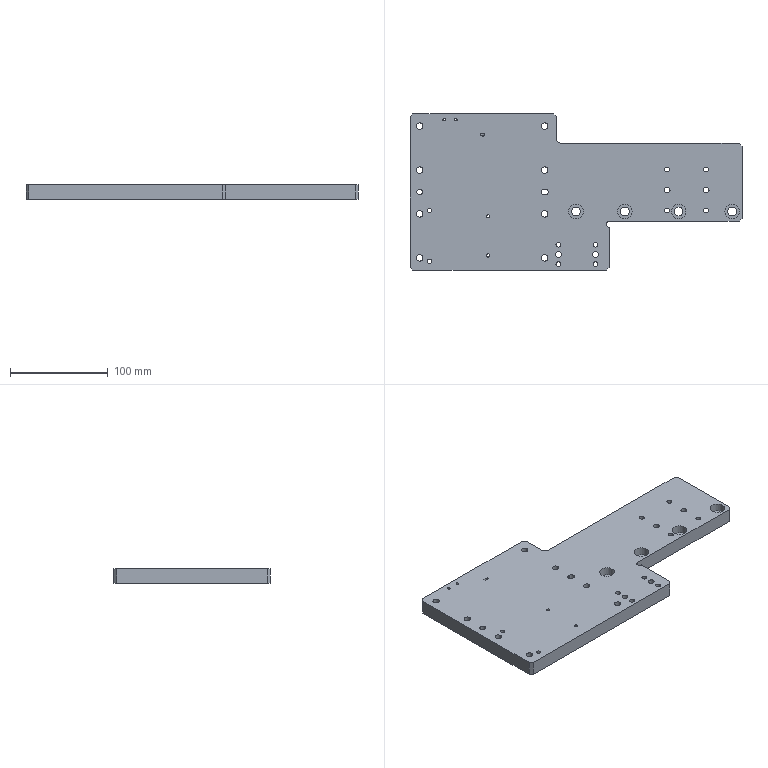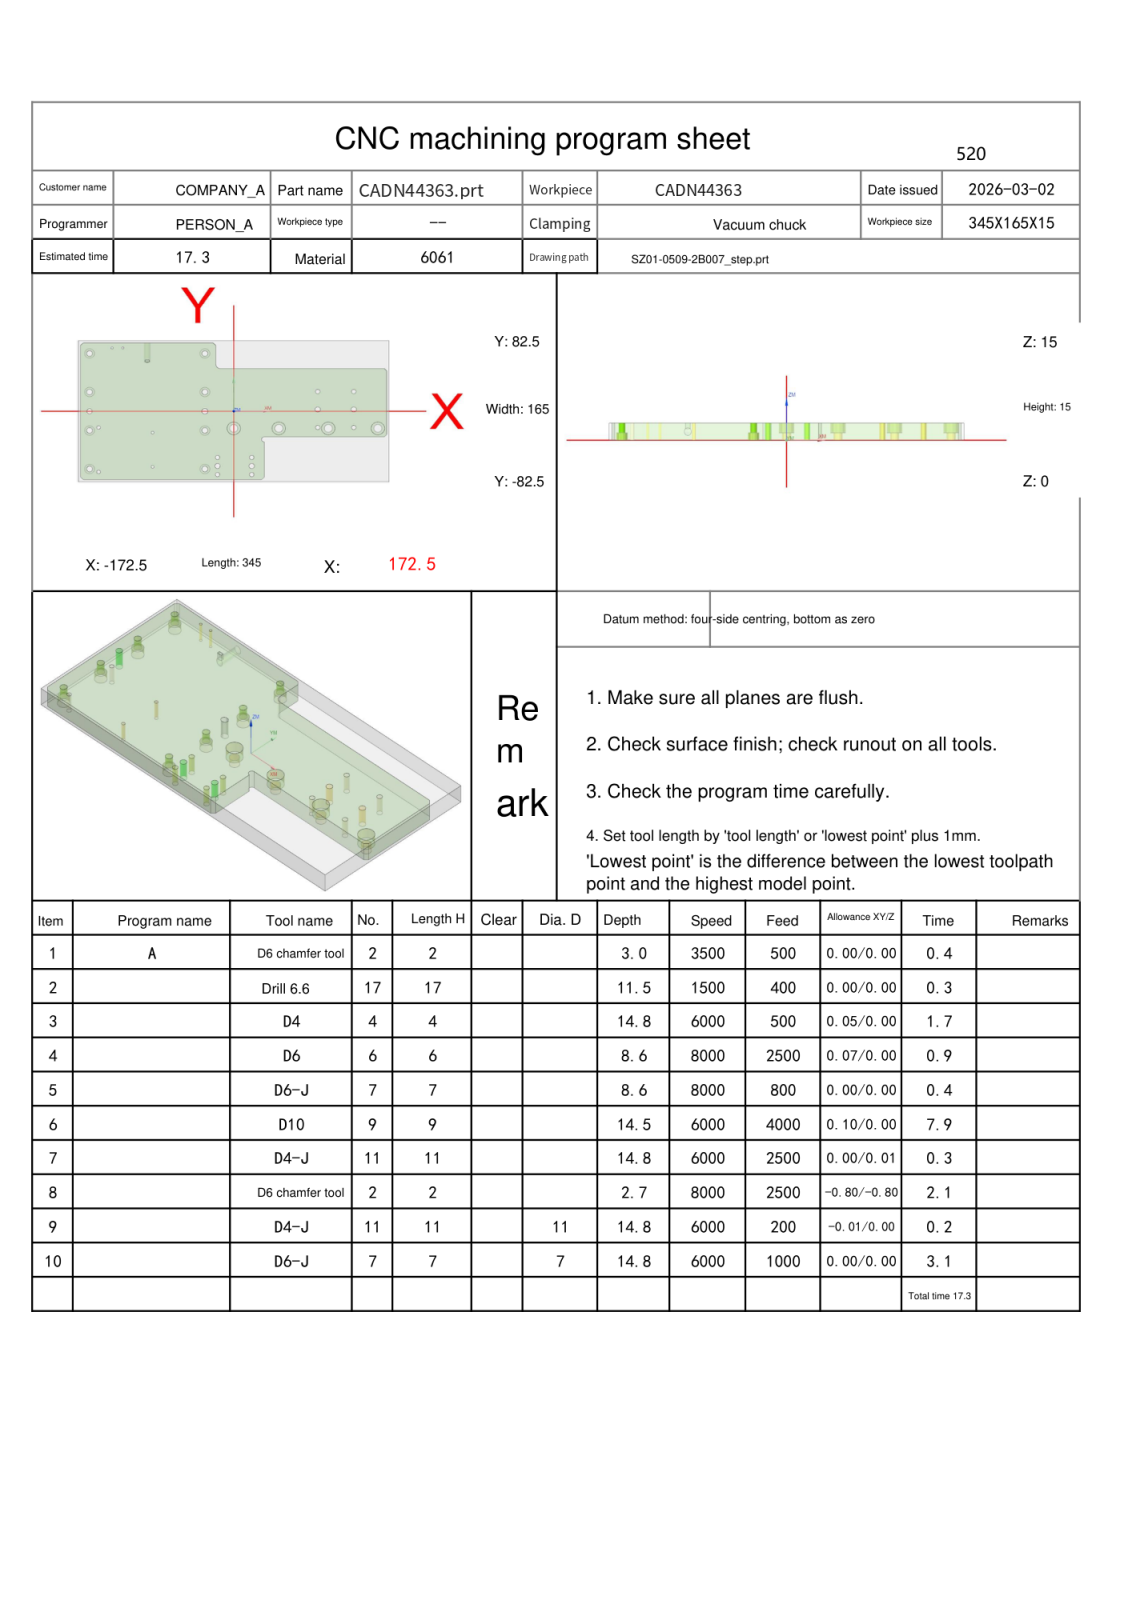NC program | NX | posted by the shop | part box 340 x 160 x 15 mm
Lines 1831 to 3961 of 3961, first 1633 of 2131 lines:
N7 T11 M06
(D4-J  D=4. R=0. H=11 ce=0.00 di=0.01)
G00 G90 G54 X39.452 Y-32.6 M03 S6000
G43 H11 Z65.
M08
Z15.304
G01 X39.451 Y-32.593 Z15.218 F2000.
X39.448 Y-32.574 Z15.14
X39.443 Y-32.545 Z15.07
X39.434 Y-32.506 Z15.008
X39.424 Y-32.461 Z14.952
X39.41 Y-32.41 Z14.903
X39.393 Y-32.356 Z14.861
X39.372 Y-32.3 Z14.824
X39.348 Y-32.244 Z14.793
X39.319 Y-32.19 Z14.767
X39.287 Y-32.139 Z14.746
X39.249 Y-32.094 Z14.73
X39.208 Y-32.055 Z14.718
X39.161 Y-32.026 Z14.71
X39.109 Y-32.007 Z14.705
X39.052 Y-32. Z14.704
X34. F2500.
G03 X33. Y-33. I0.0 J-1.
X34. Y-34. I1. J0.0
G02 X35.996 Y-35.879 I0.0 J-2.
G01 X36.015 Y-35.919 Z14.703
X36.063 Y-35.933 Z14.701
X36.136 Y-35.922 Z14.696
X36.231 Y-35.888 Z14.691
X36.344 Y-35.834 Z14.684
X36.473 Y-35.762 Z14.676
X36.615 Y-35.674 Z14.667
X36.765 Y-35.572 Z14.657
X37.001 Y-35.394 Z14.641
X37.233 Y-35.202 Z14.624
X37.561 Y-34.893 Z14.597
X37.866 Y-34.56 Z14.57
X38.147 Y-34.204 Z14.542
X38.404 Y-33.826 Z14.515
X38.635 Y-33.429 Z14.488
X38.774 Y-33.153 Z14.471
X38.858 Y-32.97 Z14.46
X38.971 Y-32.701 Z14.445
X39.03 Y-32.537 Z14.436
X39.076 Y-32.388 Z14.428
X39.107 Y-32.259 Z14.421
X39.121 Y-32.151 Z14.416
X39.118 Y-32.07 Z14.411
X39.096 Y-32.018 Z14.409
X39.052 Y-32. Z14.408
X34.
G03 X33. Y-33. I0.0 J-1.
X34. Y-34. I1. J0.0
G02 X35.996 Y-35.879 I0.0 J-2.
G01 X36.015 Y-35.919 Z14.407
X36.063 Y-35.933 Z14.405
X36.136 Y-35.922 Z14.4
X36.231 Y-35.888 Z14.395
X36.344 Y-35.834 Z14.388
X36.473 Y-35.762 Z14.38
X36.615 Y-35.674 Z14.371
X36.765 Y-35.572 Z14.361
X37.001 Y-35.394 Z14.345
X37.233 Y-35.202 Z14.328
X37.561 Y-34.893 Z14.301
X37.866 Y-34.56 Z14.274
X38.147 Y-34.204 Z14.246
X38.404 Y-33.826 Z14.219
X38.635 Y-33.429 Z14.192
X38.774 Y-33.153 Z14.175
X38.858 Y-32.97 Z14.164
X38.971 Y-32.701 Z14.149
X39.03 Y-32.537 Z14.14
X39.076 Y-32.388 Z14.132
X39.107 Y-32.259 Z14.125
X39.121 Y-32.151 Z14.12
X39.118 Y-32.07 Z14.115
X39.096 Y-32.018 Z14.113
X39.052 Y-32. Z14.112
X34.
G03 X33. Y-33. I0.0 J-1.
X34. Y-34. I1. J0.0
G02 X35.996 Y-35.879 I0.0 J-2.
G01 X36.015 Y-35.919 Z14.111
X36.063 Y-35.933 Z14.109
X36.136 Y-35.922 Z14.104
X36.231 Y-35.888 Z14.099
X36.344 Y-35.834 Z14.092
X36.473 Y-35.762 Z14.084
X36.615 Y-35.674 Z14.075
X36.765 Y-35.572 Z14.065
X37.001 Y-35.394 Z14.049
X37.233 Y-35.202 Z14.032
X37.561 Y-34.893 Z14.005
X37.866 Y-34.56 Z13.978
X38.147 Y-34.204 Z13.95
X38.404 Y-33.826 Z13.923
X38.635 Y-33.429 Z13.896
X38.774 Y-33.153 Z13.879
X38.858 Y-32.97 Z13.868
X38.971 Y-32.701 Z13.853
X39.03 Y-32.537 Z13.844
X39.076 Y-32.388 Z13.836
X39.107 Y-32.259 Z13.829
X39.121 Y-32.151 Z13.824
X39.118 Y-32.07 Z13.819
X39.096 Y-32.018 Z13.817
X39.052 Y-32. Z13.816
X34.
G03 X33. Y-33. I0.0 J-1.
X34. Y-34. I1. J0.0
G02 X35.996 Y-35.879 I0.0 J-2.
G01 X36.015 Y-35.919 Z13.815
X36.063 Y-35.933 Z13.813
X36.136 Y-35.922 Z13.808
X36.231 Y-35.888 Z13.803
X36.344 Y-35.834 Z13.796
X36.473 Y-35.762 Z13.788
X36.615 Y-35.674 Z13.779
X36.765 Y-35.572 Z13.769
X37.001 Y-35.394 Z13.753
X37.233 Y-35.202 Z13.736
X37.561 Y-34.893 Z13.709
X37.866 Y-34.56 Z13.682
X38.147 Y-34.204 Z13.654
X38.404 Y-33.826 Z13.627
X38.635 Y-33.429 Z13.6
X38.774 Y-33.153 Z13.583
X38.858 Y-32.97 Z13.572
X38.971 Y-32.701 Z13.557
X39.03 Y-32.537 Z13.548
X39.076 Y-32.388 Z13.54
X39.107 Y-32.259 Z13.533
X39.121 Y-32.151 Z13.528
X39.118 Y-32.07 Z13.523
X39.096 Y-32.018 Z13.521
X39.052 Y-32. Z13.52
X34.
G03 X33. Y-33. I0.0 J-1.
X34. Y-34. I1. J0.0
G02 X35.996 Y-35.879 I0.0 J-2.
G01 X36.015 Y-35.919 Z13.519
X36.063 Y-35.933 Z13.517
X36.136 Y-35.922 Z13.512
X36.231 Y-35.888 Z13.507
X36.344 Y-35.834 Z13.5
X36.473 Y-35.762 Z13.492
X36.615 Y-35.674 Z13.483
X36.765 Y-35.572 Z13.473
X37.001 Y-35.394 Z13.457
X37.233 Y-35.202 Z13.44
X37.561 Y-34.893 Z13.413
X37.866 Y-34.56 Z13.386
X38.147 Y-34.204 Z13.358
X38.404 Y-33.826 Z13.331
X38.635 Y-33.429 Z13.304
X38.774 Y-33.153 Z13.287
X38.858 Y-32.97 Z13.276
X38.971 Y-32.701 Z13.261
X39.03 Y-32.537 Z13.252
X39.076 Y-32.388 Z13.244
X39.107 Y-32.259 Z13.237
X39.121 Y-32.151 Z13.232
X39.118 Y-32.07 Z13.227
X39.096 Y-32.018 Z13.225
X39.052 Y-32. Z13.224
X34.
G03 X33. Y-33. I0.0 J-1.
X34. Y-34. I1. J0.0
G02 X35.996 Y-35.879 I0.0 J-2.
G01 X36.015 Y-35.919 Z13.223
X36.063 Y-35.933 Z13.221
X36.136 Y-35.922 Z13.216
X36.231 Y-35.888 Z13.211
X36.344 Y-35.834 Z13.204
X36.473 Y-35.762 Z13.196
X36.615 Y-35.674 Z13.187
X36.765 Y-35.572 Z13.177
X37.001 Y-35.394 Z13.161
X37.233 Y-35.202 Z13.144
X37.561 Y-34.893 Z13.117
X37.866 Y-34.56 Z13.09
X38.147 Y-34.204 Z13.062
X38.404 Y-33.826 Z13.035
X38.635 Y-33.429 Z13.008
X38.774 Y-33.153 Z12.991
X38.858 Y-32.97 Z12.98
X38.971 Y-32.701 Z12.965
X39.03 Y-32.537 Z12.956
X39.076 Y-32.388 Z12.948
X39.107 Y-32.259 Z12.941
X39.121 Y-32.151 Z12.936
X39.118 Y-32.07 Z12.931
X39.096 Y-32.018 Z12.929
X39.052 Y-32. Z12.928
X34.
G03 X33. Y-33. I0.0 J-1.
X34. Y-34. I1. J0.0
G02 X35.996 Y-35.879 I0.0 J-2.
G01 X36.015 Y-35.919 Z12.927
X36.063 Y-35.933 Z12.925
X36.136 Y-35.922 Z12.92
X36.231 Y-35.888 Z12.915
X36.344 Y-35.834 Z12.908
X36.473 Y-35.762 Z12.9
X36.615 Y-35.674 Z12.891
X36.765 Y-35.572 Z12.881
X37.001 Y-35.394 Z12.865
X37.233 Y-35.202 Z12.848
X37.561 Y-34.893 Z12.821
X37.866 Y-34.56 Z12.794
X38.147 Y-34.204 Z12.766
X38.404 Y-33.826 Z12.739
X38.635 Y-33.429 Z12.712
X38.774 Y-33.153 Z12.695
X38.858 Y-32.97 Z12.684
X38.971 Y-32.701 Z12.669
X39.03 Y-32.537 Z12.66
X39.076 Y-32.388 Z12.652
X39.107 Y-32.259 Z12.645
X39.121 Y-32.151 Z12.64
X39.118 Y-32.07 Z12.635
X39.096 Y-32.018 Z12.633
X39.052 Y-32. Z12.632
X34.
G03 X33. Y-33. I0.0 J-1.
X34. Y-34. I1. J0.0
G02 X35.996 Y-35.879 I0.0 J-2.
G01 X36.015 Y-35.919 Z12.631
X36.063 Y-35.933 Z12.629
X36.136 Y-35.922 Z12.624
X36.231 Y-35.888 Z12.619
X36.344 Y-35.834 Z12.612
X36.473 Y-35.762 Z12.604
X36.615 Y-35.674 Z12.595
X36.765 Y-35.572 Z12.585
X37.001 Y-35.394 Z12.569
X37.233 Y-35.202 Z12.552
X37.561 Y-34.893 Z12.525
X37.866 Y-34.56 Z12.498
X38.147 Y-34.204 Z12.47
X38.404 Y-33.826 Z12.443
X38.635 Y-33.429 Z12.416
X38.774 Y-33.153 Z12.399
X38.858 Y-32.97 Z12.388
X38.971 Y-32.701 Z12.373
X39.03 Y-32.537 Z12.364
X39.076 Y-32.388 Z12.356
X39.107 Y-32.259 Z12.349
X39.121 Y-32.151 Z12.344
X39.118 Y-32.07 Z12.339
X39.096 Y-32.018 Z12.337
X39.052 Y-32. Z12.336
X34.
G03 X33. Y-33. I0.0 J-1.
X34. Y-34. I1. J0.0
G02 X35.996 Y-35.879 I0.0 J-2.
G01 X36.015 Y-35.919 Z12.335
X36.063 Y-35.933 Z12.333
X36.136 Y-35.922 Z12.328
X36.231 Y-35.888 Z12.323
X36.344 Y-35.834 Z12.316
X36.473 Y-35.762 Z12.308
X36.615 Y-35.674 Z12.299
X36.765 Y-35.572 Z12.289
X37.001 Y-35.394 Z12.273
X37.233 Y-35.202 Z12.256
X37.561 Y-34.893 Z12.229
X37.866 Y-34.56 Z12.202
X38.147 Y-34.204 Z12.174
X38.404 Y-33.826 Z12.147
X38.635 Y-33.429 Z12.12
X38.774 Y-33.153 Z12.103
X38.858 Y-32.97 Z12.092
X38.971 Y-32.701 Z12.077
X39.03 Y-32.537 Z12.068
X39.076 Y-32.388 Z12.06
X39.107 Y-32.259 Z12.053
X39.121 Y-32.151 Z12.048
X39.118 Y-32.07 Z12.043
X39.096 Y-32.018 Z12.041
X39.052 Y-32. Z12.04
X34.
G03 X33. Y-33. I0.0 J-1.
X34. Y-34. I1. J0.0
G02 X35.996 Y-35.879 I0.0 J-2.
G01 X36.015 Y-35.919 Z12.039
X36.063 Y-35.933 Z12.037
X36.136 Y-35.922 Z12.032
X36.231 Y-35.888 Z12.027
X36.344 Y-35.834 Z12.02
X36.473 Y-35.762 Z12.012
X36.615 Y-35.674 Z12.003
X36.765 Y-35.572 Z11.993
X37.001 Y-35.394 Z11.977
X37.233 Y-35.202 Z11.96
X37.561 Y-34.893 Z11.933
X37.866 Y-34.56 Z11.906
X38.147 Y-34.204 Z11.878
X38.404 Y-33.826 Z11.851
X38.635 Y-33.429 Z11.824
X38.774 Y-33.153 Z11.807
X38.858 Y-32.97 Z11.796
X38.971 Y-32.701 Z11.781
X39.03 Y-32.537 Z11.772
X39.076 Y-32.388 Z11.764
X39.107 Y-32.259 Z11.757
X39.121 Y-32.151 Z11.752
X39.118 Y-32.07 Z11.747
X39.096 Y-32.018 Z11.745
X39.052 Y-32. Z11.744
X34.
G03 X33. Y-33. I0.0 J-1.
X34. Y-34. I1. J0.0
G02 X35.996 Y-35.879 I0.0 J-2.
G01 X36.015 Y-35.919 Z11.743
X36.063 Y-35.933 Z11.741
X36.136 Y-35.922 Z11.736
X36.231 Y-35.888 Z11.731
X36.344 Y-35.834 Z11.724
X36.473 Y-35.762 Z11.716
X36.615 Y-35.674 Z11.707
X36.765 Y-35.572 Z11.697
X37.001 Y-35.394 Z11.681
X37.233 Y-35.202 Z11.664
X37.561 Y-34.893 Z11.637
X37.866 Y-34.56 Z11.61
X38.147 Y-34.204 Z11.582
X38.404 Y-33.826 Z11.555
X38.635 Y-33.429 Z11.528
X38.774 Y-33.153 Z11.511
X38.858 Y-32.97 Z11.5
X38.971 Y-32.701 Z11.485
X39.03 Y-32.537 Z11.476
X39.076 Y-32.388 Z11.468
X39.107 Y-32.259 Z11.461
X39.121 Y-32.151 Z11.456
X39.118 Y-32.07 Z11.451
X39.096 Y-32.018 Z11.449
X39.052 Y-32. Z11.448
X34.
G03 X33. Y-33. I0.0 J-1.
X34. Y-34. I1. J0.0
G02 X35.996 Y-35.879 I0.0 J-2.
G01 X36.015 Y-35.919 Z11.447
X36.063 Y-35.933 Z11.445
X36.136 Y-35.922 Z11.44
X36.231 Y-35.888 Z11.435
X36.344 Y-35.834 Z11.428
X36.473 Y-35.762 Z11.42
X36.615 Y-35.674 Z11.411
X36.765 Y-35.572 Z11.401
X37.001 Y-35.394 Z11.385
X37.233 Y-35.202 Z11.368
X37.561 Y-34.893 Z11.341
X37.866 Y-34.56 Z11.314
X38.147 Y-34.204 Z11.286
X38.404 Y-33.826 Z11.259
X38.635 Y-33.429 Z11.232
X38.774 Y-33.153 Z11.215
X38.858 Y-32.97 Z11.204
X38.971 Y-32.701 Z11.189
X39.03 Y-32.537 Z11.18
X39.076 Y-32.388 Z11.172
X39.107 Y-32.259 Z11.165
X39.121 Y-32.151 Z11.16
X39.118 Y-32.07 Z11.155
X39.096 Y-32.018 Z11.153
X39.052 Y-32. Z11.152
X34.
G03 X33. Y-33. I0.0 J-1.
X34. Y-34. I1. J0.0
G02 X35.996 Y-35.879 I0.0 J-2.
G01 X36.015 Y-35.919 Z11.151
X36.063 Y-35.933 Z11.149
X36.136 Y-35.922 Z11.144
X36.231 Y-35.888 Z11.139
X36.344 Y-35.834 Z11.132
X36.473 Y-35.762 Z11.124
X36.615 Y-35.674 Z11.115
X36.765 Y-35.572 Z11.105
X37.001 Y-35.394 Z11.089
X37.233 Y-35.202 Z11.072
X37.561 Y-34.893 Z11.045
X37.866 Y-34.56 Z11.018
X38.147 Y-34.204 Z10.99
X38.404 Y-33.826 Z10.963
X38.635 Y-33.429 Z10.936
X38.774 Y-33.153 Z10.919
X38.858 Y-32.97 Z10.908
X38.971 Y-32.701 Z10.893
X39.03 Y-32.537 Z10.884
X39.076 Y-32.388 Z10.876
X39.107 Y-32.259 Z10.869
X39.121 Y-32.151 Z10.864
X39.118 Y-32.07 Z10.859
X39.096 Y-32.018 Z10.857
X39.052 Y-32. Z10.856
X34.
G03 X33. Y-33. I0.0 J-1.
X34. Y-34. I1. J0.0
G02 X35.996 Y-35.879 I0.0 J-2.
G01 X36.015 Y-35.919 Z10.855
X36.063 Y-35.933 Z10.853
X36.136 Y-35.922 Z10.848
X36.231 Y-35.888 Z10.843
X36.344 Y-35.834 Z10.836
X36.473 Y-35.762 Z10.828
X36.615 Y-35.674 Z10.819
X36.765 Y-35.572 Z10.809
X37.001 Y-35.394 Z10.793
X37.233 Y-35.202 Z10.776
X37.561 Y-34.893 Z10.749
X37.866 Y-34.56 Z10.722
X38.147 Y-34.204 Z10.694
X38.404 Y-33.826 Z10.667
X38.635 Y-33.429 Z10.64
X38.774 Y-33.153 Z10.623
X38.858 Y-32.97 Z10.612
X38.971 Y-32.701 Z10.597
X39.03 Y-32.537 Z10.588
X39.076 Y-32.388 Z10.58
X39.107 Y-32.259 Z10.573
X39.121 Y-32.151 Z10.568
X39.118 Y-32.07 Z10.563
X39.096 Y-32.018 Z10.561
X39.052 Y-32. Z10.56
X34.
G03 X33. Y-33. I0.0 J-1.
X34. Y-34. I1. J0.0
G02 X35.996 Y-35.879 I0.0 J-2.
G01 X36.015 Y-35.919 Z10.559
X36.063 Y-35.933 Z10.557
X36.136 Y-35.922 Z10.552
X36.231 Y-35.888 Z10.547
X36.344 Y-35.834 Z10.54
X36.473 Y-35.762 Z10.532
X36.615 Y-35.674 Z10.523
X36.765 Y-35.572 Z10.513
X37.001 Y-35.394 Z10.497
X37.233 Y-35.202 Z10.48
X37.561 Y-34.893 Z10.453
X37.866 Y-34.56 Z10.426
X38.147 Y-34.204 Z10.398
X38.404 Y-33.826 Z10.371
X38.635 Y-33.429 Z10.344
X38.774 Y-33.153 Z10.327
X38.858 Y-32.97 Z10.316
X38.971 Y-32.701 Z10.301
X39.03 Y-32.537 Z10.292
X39.076 Y-32.388 Z10.284
X39.107 Y-32.259 Z10.277
X39.121 Y-32.151 Z10.272
X39.118 Y-32.07 Z10.267
X39.096 Y-32.018 Z10.265
X39.052 Y-32. Z10.264
X34.
G03 X33. Y-33. I0.0 J-1.
X34. Y-34. I1. J0.0
G02 X35.996 Y-35.879 I0.0 J-2.
G01 X36.015 Y-35.919 Z10.263
X36.063 Y-35.933 Z10.261
X36.136 Y-35.922 Z10.256
X36.231 Y-35.888 Z10.251
X36.344 Y-35.834 Z10.244
X36.473 Y-35.762 Z10.236
X36.615 Y-35.674 Z10.227
X36.765 Y-35.572 Z10.217
X37.001 Y-35.394 Z10.201
X37.233 Y-35.202 Z10.184
X37.561 Y-34.893 Z10.157
X37.866 Y-34.56 Z10.13
X38.147 Y-34.204 Z10.102
X38.404 Y-33.826 Z10.075
X38.635 Y-33.429 Z10.048
X38.774 Y-33.153 Z10.031
X38.858 Y-32.97 Z10.02
X38.971 Y-32.701 Z10.005
X39.03 Y-32.537 Z9.996
X39.076 Y-32.388 Z9.988
X39.107 Y-32.259 Z9.981
X39.121 Y-32.151 Z9.976
X39.118 Y-32.07 Z9.971
X39.096 Y-32.018 Z9.969
X39.052 Y-32. Z9.968
X34.
G03 X33. Y-33. I0.0 J-1.
X34. Y-34. I1. J0.0
G02 X35.996 Y-35.879 I0.0 J-2.
G01 X36.015 Y-35.919 Z9.967
X36.063 Y-35.933 Z9.965
X36.136 Y-35.922 Z9.96
X36.231 Y-35.888 Z9.955
X36.344 Y-35.834 Z9.948
X36.473 Y-35.762 Z9.94
X36.615 Y-35.674 Z9.931
X36.765 Y-35.572 Z9.921
X37.001 Y-35.394 Z9.905
X37.233 Y-35.202 Z9.888
X37.561 Y-34.893 Z9.861
X37.866 Y-34.56 Z9.834
X38.147 Y-34.204 Z9.806
X38.404 Y-33.826 Z9.779
X38.635 Y-33.429 Z9.752
X38.774 Y-33.153 Z9.735
X38.858 Y-32.97 Z9.724
X38.971 Y-32.701 Z9.709
X39.03 Y-32.537 Z9.7
X39.076 Y-32.388 Z9.692
X39.107 Y-32.259 Z9.685
X39.121 Y-32.151 Z9.68
X39.118 Y-32.07 Z9.675
X39.096 Y-32.018 Z9.673
X39.052 Y-32. Z9.672
X34.
G03 X33. Y-33. I0.0 J-1.
X34. Y-34. I1. J0.0
G02 X35.996 Y-35.879 I0.0 J-2.
G01 X36.015 Y-35.919 Z9.671
X36.063 Y-35.933 Z9.669
X36.136 Y-35.922 Z9.664
X36.231 Y-35.888 Z9.659
X36.344 Y-35.834 Z9.652
X36.473 Y-35.762 Z9.644
X36.615 Y-35.674 Z9.635
X36.765 Y-35.572 Z9.625
X37.001 Y-35.394 Z9.609
X37.233 Y-35.202 Z9.592
X37.561 Y-34.893 Z9.565
X37.866 Y-34.56 Z9.538
X38.147 Y-34.204 Z9.51
X38.404 Y-33.826 Z9.483
X38.635 Y-33.429 Z9.456
X38.774 Y-33.153 Z9.439
X38.858 Y-32.97 Z9.428
X38.971 Y-32.701 Z9.413
X39.03 Y-32.537 Z9.404
X39.076 Y-32.388 Z9.396
X39.107 Y-32.259 Z9.389
X39.121 Y-32.151 Z9.384
X39.118 Y-32.07 Z9.379
X39.096 Y-32.018 Z9.377
X39.052 Y-32. Z9.376
X34.
G03 X33. Y-33. I0.0 J-1.
X34. Y-34. I1. J0.0
G02 X35.996 Y-35.879 I0.0 J-2.
G01 X36.015 Y-35.919 Z9.375
X36.063 Y-35.933 Z9.373
X36.136 Y-35.922 Z9.368
X36.231 Y-35.888 Z9.363
X36.344 Y-35.834 Z9.356
X36.473 Y-35.762 Z9.348
X36.615 Y-35.674 Z9.339
X36.765 Y-35.572 Z9.329
X37.001 Y-35.394 Z9.313
X37.233 Y-35.202 Z9.296
X37.561 Y-34.893 Z9.269
X37.866 Y-34.56 Z9.242
X38.147 Y-34.204 Z9.214
X38.404 Y-33.826 Z9.187
X38.635 Y-33.429 Z9.16
X38.774 Y-33.153 Z9.143
X38.858 Y-32.97 Z9.132
X38.971 Y-32.701 Z9.117
X39.03 Y-32.537 Z9.108
X39.076 Y-32.388 Z9.1
X39.107 Y-32.259 Z9.093
X39.121 Y-32.151 Z9.088
X39.118 Y-32.07 Z9.083
X39.096 Y-32.018 Z9.081
X39.052 Y-32. Z9.08
X34.
G03 X33. Y-33. I0.0 J-1.
X34. Y-34. I1. J0.0
G02 X35.996 Y-35.879 I0.0 J-2.
G01 X36.015 Y-35.919 Z9.079
X36.063 Y-35.933 Z9.077
X36.136 Y-35.922 Z9.072
X36.231 Y-35.888 Z9.067
X36.344 Y-35.834 Z9.06
X36.473 Y-35.762 Z9.052
X36.615 Y-35.674 Z9.043
X36.765 Y-35.572 Z9.033
X37.001 Y-35.394 Z9.017
X37.233 Y-35.202 Z9.
X37.561 Y-34.893 Z8.973
X37.866 Y-34.56 Z8.946
X38.147 Y-34.204 Z8.918
X38.404 Y-33.826 Z8.891
X38.635 Y-33.429 Z8.864
X38.774 Y-33.153 Z8.847
X38.858 Y-32.97 Z8.836
X38.971 Y-32.701 Z8.821
X39.03 Y-32.537 Z8.812
X39.076 Y-32.388 Z8.804
X39.107 Y-32.259 Z8.797
X39.121 Y-32.151 Z8.792
X39.118 Y-32.07 Z8.787
X39.096 Y-32.018 Z8.785
X39.052 Y-32. Z8.784
X34.
G03 X33. Y-33. I0.0 J-1.
X34. Y-34. I1. J0.0
G02 X35.996 Y-35.879 I0.0 J-2.
G01 X36.015 Y-35.919 Z8.783
X36.063 Y-35.933 Z8.781
X36.136 Y-35.922 Z8.776
X36.231 Y-35.888 Z8.771
X36.344 Y-35.834 Z8.764
X36.473 Y-35.762 Z8.756
X36.615 Y-35.674 Z8.747
X36.765 Y-35.572 Z8.737
X37.001 Y-35.394 Z8.721
X37.233 Y-35.202 Z8.704
X37.561 Y-34.893 Z8.677
X37.866 Y-34.56 Z8.65
X38.147 Y-34.204 Z8.622
X38.404 Y-33.826 Z8.595
X38.635 Y-33.429 Z8.568
X38.774 Y-33.153 Z8.551
X38.858 Y-32.97 Z8.54
X38.971 Y-32.701 Z8.525
X39.03 Y-32.537 Z8.516
X39.076 Y-32.388 Z8.508
X39.107 Y-32.259 Z8.501
X39.121 Y-32.151 Z8.496
X39.118 Y-32.07 Z8.491
X39.096 Y-32.018 Z8.489
X39.052 Y-32. Z8.488
X34.
G03 X33. Y-33. I0.0 J-1.
X34. Y-34. I1. J0.0
G02 X35.996 Y-35.879 I0.0 J-2.
G01 X36.015 Y-35.919 Z8.487
X36.063 Y-35.933 Z8.485
X36.136 Y-35.922 Z8.48
X36.231 Y-35.888 Z8.475
X36.344 Y-35.834 Z8.468
X36.473 Y-35.762 Z8.46
X36.615 Y-35.674 Z8.451
X36.765 Y-35.572 Z8.441
X37.001 Y-35.394 Z8.425
X37.233 Y-35.202 Z8.408
X37.561 Y-34.893 Z8.381
X37.866 Y-34.56 Z8.354
X38.147 Y-34.204 Z8.326
X38.404 Y-33.826 Z8.299
X38.635 Y-33.429 Z8.272
X38.774 Y-33.153 Z8.255
X38.858 Y-32.97 Z8.244
X38.971 Y-32.701 Z8.229
X39.03 Y-32.537 Z8.22
X39.076 Y-32.388 Z8.212
X39.107 Y-32.259 Z8.205
X39.121 Y-32.151 Z8.2
X39.118 Y-32.07 Z8.195
X39.096 Y-32.018 Z8.193
X39.052 Y-32. Z8.192
X34.
G03 X33. Y-33. I0.0 J-1.
X34. Y-34. I1. J0.0
G02 X35.996 Y-35.879 I0.0 J-2.
G01 X36.015 Y-35.919 Z8.191
X36.063 Y-35.933 Z8.189
X36.136 Y-35.922 Z8.184
X36.231 Y-35.888 Z8.179
X36.344 Y-35.834 Z8.172
X36.473 Y-35.762 Z8.164
X36.615 Y-35.674 Z8.155
X36.765 Y-35.572 Z8.145
X37.001 Y-35.394 Z8.129
X37.233 Y-35.202 Z8.112
X37.561 Y-34.893 Z8.085
X37.866 Y-34.56 Z8.058
X38.147 Y-34.204 Z8.03
X38.404 Y-33.826 Z8.003
X38.635 Y-33.429 Z7.976
X38.774 Y-33.153 Z7.959
X38.858 Y-32.97 Z7.948
X38.971 Y-32.701 Z7.933
X39.03 Y-32.537 Z7.924
X39.076 Y-32.388 Z7.916
X39.107 Y-32.259 Z7.909
X39.121 Y-32.151 Z7.904
X39.118 Y-32.07 Z7.899
X39.096 Y-32.018 Z7.897
X39.052 Y-32. Z7.896
X34.
G03 X33. Y-33. I0.0 J-1.
X34. Y-34. I1. J0.0
G02 X35.996 Y-35.879 I0.0 J-2.
G01 X36.015 Y-35.919 Z7.895
X36.063 Y-35.933 Z7.893
X36.136 Y-35.922 Z7.888
X36.231 Y-35.888 Z7.883
X36.344 Y-35.834 Z7.876
X36.473 Y-35.762 Z7.868
X36.615 Y-35.674 Z7.859
X36.765 Y-35.572 Z7.849
X37.001 Y-35.394 Z7.833
X37.233 Y-35.202 Z7.816
X37.561 Y-34.893 Z7.789
X37.866 Y-34.56 Z7.762
X38.147 Y-34.204 Z7.734
X38.404 Y-33.826 Z7.707
X38.635 Y-33.429 Z7.68
X38.774 Y-33.153 Z7.663
X38.858 Y-32.97 Z7.652
X38.971 Y-32.701 Z7.637
X39.03 Y-32.537 Z7.628
X39.076 Y-32.388 Z7.62
X39.107 Y-32.259 Z7.613
X39.121 Y-32.151 Z7.608
X39.118 Y-32.07 Z7.603
X39.096 Y-32.018 Z7.601
X39.052 Y-32. Z7.6
X34.
G03 X33. Y-33. I0.0 J-1.
X34. Y-34. I1. J0.0
G02 X35.996 Y-35.879 I0.0 J-2.
G01 X36.015 Y-35.919 Z7.599
X36.063 Y-35.933 Z7.597
X36.136 Y-35.922 Z7.592
X36.231 Y-35.888 Z7.587
X36.344 Y-35.834 Z7.58
X36.473 Y-35.762 Z7.572
X36.615 Y-35.674 Z7.563
X36.765 Y-35.572 Z7.553
X37.001 Y-35.394 Z7.537
X37.233 Y-35.202 Z7.52
X37.561 Y-34.893 Z7.493
X37.866 Y-34.56 Z7.466
X38.147 Y-34.204 Z7.438
X38.404 Y-33.826 Z7.411
X38.635 Y-33.429 Z7.384
X38.774 Y-33.153 Z7.367
X38.858 Y-32.97 Z7.356
X38.971 Y-32.701 Z7.341
X39.03 Y-32.537 Z7.332
X39.076 Y-32.388 Z7.324
X39.107 Y-32.259 Z7.317
X39.121 Y-32.151 Z7.312
X39.118 Y-32.07 Z7.307
X39.096 Y-32.018 Z7.305
X39.052 Y-32. Z7.304
X34.
G03 X33. Y-33. I0.0 J-1.
X34. Y-34. I1. J0.0
G02 X35.996 Y-35.879 I0.0 J-2.
G01 X36.015 Y-35.919 Z7.303
X36.063 Y-35.933 Z7.301
X36.136 Y-35.922 Z7.296
X36.231 Y-35.888 Z7.291
X36.344 Y-35.834 Z7.284
X36.473 Y-35.762 Z7.276
X36.615 Y-35.674 Z7.267
X36.765 Y-35.572 Z7.257
X37.001 Y-35.394 Z7.241
X37.233 Y-35.202 Z7.224
X37.561 Y-34.893 Z7.197
X37.866 Y-34.56 Z7.17
X38.147 Y-34.204 Z7.142
X38.404 Y-33.826 Z7.115
X38.635 Y-33.429 Z7.088
X38.774 Y-33.153 Z7.071
X38.858 Y-32.97 Z7.06
X38.971 Y-32.701 Z7.045
X39.03 Y-32.537 Z7.036
X39.076 Y-32.388 Z7.028
X39.107 Y-32.259 Z7.021
X39.121 Y-32.151 Z7.016
X39.118 Y-32.07 Z7.011
X39.096 Y-32.018 Z7.009
X39.052 Y-32. Z7.008
X34.
G03 X33. Y-33. I0.0 J-1.
X34. Y-34. I1. J0.0
G02 X35.996 Y-35.879 I0.0 J-2.
G01 X36.015 Y-35.919 Z7.007
X36.063 Y-35.933 Z7.005
X36.136 Y-35.922 Z7.
X36.231 Y-35.888 Z6.995
X36.344 Y-35.834 Z6.988
X36.473 Y-35.762 Z6.98
X36.615 Y-35.674 Z6.971
X36.765 Y-35.572 Z6.961
X37.001 Y-35.394 Z6.945
X37.233 Y-35.202 Z6.928
X37.561 Y-34.893 Z6.901
X37.866 Y-34.56 Z6.874
X38.147 Y-34.204 Z6.846
X38.404 Y-33.826 Z6.819
X38.635 Y-33.429 Z6.792
X38.774 Y-33.153 Z6.775
X38.858 Y-32.97 Z6.764
X38.971 Y-32.701 Z6.749
X39.03 Y-32.537 Z6.74
X39.076 Y-32.388 Z6.732
X39.107 Y-32.259 Z6.725
X39.121 Y-32.151 Z6.72
X39.118 Y-32.07 Z6.715
X39.096 Y-32.018 Z6.713
X39.052 Y-32. Z6.712
X34.
G03 X33. Y-33. I0.0 J-1.
X34. Y-34. I1. J0.0
G02 X35.996 Y-35.879 I0.0 J-2.
G01 X36.015 Y-35.919 Z6.711
X36.063 Y-35.933 Z6.709
X36.136 Y-35.922 Z6.704
X36.231 Y-35.888 Z6.699
X36.344 Y-35.834 Z6.692
X36.473 Y-35.762 Z6.684
X36.615 Y-35.674 Z6.675
X36.765 Y-35.572 Z6.665
X37.001 Y-35.394 Z6.649
X37.233 Y-35.202 Z6.632
X37.561 Y-34.893 Z6.605
X37.866 Y-34.56 Z6.578
X38.147 Y-34.204 Z6.55
X38.404 Y-33.826 Z6.523
X38.635 Y-33.429 Z6.496
X38.774 Y-33.153 Z6.479
X38.858 Y-32.97 Z6.468
X38.971 Y-32.701 Z6.453
X39.03 Y-32.537 Z6.444
X39.076 Y-32.388 Z6.436
X39.107 Y-32.259 Z6.429
X39.121 Y-32.151 Z6.424
X39.118 Y-32.07 Z6.419
X39.096 Y-32.018 Z6.417
X39.052 Y-32. Z6.416
X34.
G03 X33. Y-33. I0.0 J-1.
X34. Y-34. I1. J0.0
G02 X35.996 Y-35.879 I0.0 J-2.
G01 X36.015 Y-35.919 Z6.415
X36.063 Y-35.933 Z6.413
X36.136 Y-35.922 Z6.408
X36.231 Y-35.888 Z6.403
X36.344 Y-35.834 Z6.396
X36.473 Y-35.762 Z6.388
X36.615 Y-35.674 Z6.379
X36.765 Y-35.572 Z6.369
X37.001 Y-35.394 Z6.353
X37.233 Y-35.202 Z6.336
X37.561 Y-34.893 Z6.309
X37.866 Y-34.56 Z6.282
X38.147 Y-34.204 Z6.254
X38.404 Y-33.826 Z6.227
X38.635 Y-33.429 Z6.2
X38.774 Y-33.153 Z6.183
X38.858 Y-32.97 Z6.172
X38.971 Y-32.701 Z6.157
X39.03 Y-32.537 Z6.148
X39.076 Y-32.388 Z6.14
X39.107 Y-32.259 Z6.133
X39.121 Y-32.151 Z6.128
X39.118 Y-32.07 Z6.123
X39.096 Y-32.018 Z6.121
X39.052 Y-32. Z6.12
X34.
G03 X33. Y-33. I0.0 J-1.
X34. Y-34. I1. J0.0
G02 X35.996 Y-35.879 I0.0 J-2.
G01 X36.015 Y-35.919 Z6.119
X36.063 Y-35.933 Z6.117
X36.136 Y-35.922 Z6.112
X36.231 Y-35.888 Z6.107
X36.344 Y-35.834 Z6.1
X36.473 Y-35.762 Z6.092
X36.615 Y-35.674 Z6.083
X36.765 Y-35.572 Z6.073
X37.001 Y-35.394 Z6.057
X37.233 Y-35.202 Z6.04
X37.561 Y-34.893 Z6.013
X37.866 Y-34.56 Z5.986
X38.147 Y-34.204 Z5.958
X38.404 Y-33.826 Z5.931
X38.635 Y-33.429 Z5.904
X38.774 Y-33.153 Z5.887
X38.858 Y-32.97 Z5.876
X38.971 Y-32.701 Z5.861
X39.03 Y-32.537 Z5.852
X39.076 Y-32.388 Z5.844
X39.107 Y-32.259 Z5.837
X39.121 Y-32.151 Z5.832
X39.118 Y-32.07 Z5.827
X39.096 Y-32.018 Z5.825
X39.052 Y-32. Z5.824
X34.
G03 X33. Y-33. I0.0 J-1.
X34. Y-34. I1. J0.0
G02 X35.996 Y-35.879 I0.0 J-2.
G01 X36.015 Y-35.919 Z5.823
X36.063 Y-35.933 Z5.821
X36.136 Y-35.922 Z5.816
X36.231 Y-35.888 Z5.811
X36.344 Y-35.834 Z5.804
X36.473 Y-35.762 Z5.796
X36.615 Y-35.674 Z5.787
X36.765 Y-35.572 Z5.777
X37.001 Y-35.394 Z5.761
X37.233 Y-35.202 Z5.744
X37.561 Y-34.893 Z5.717
X37.866 Y-34.56 Z5.69
X38.147 Y-34.204 Z5.662
X38.404 Y-33.826 Z5.635
X38.635 Y-33.429 Z5.608
X38.774 Y-33.153 Z5.591
X38.858 Y-32.97 Z5.58
X38.971 Y-32.701 Z5.565
X39.03 Y-32.537 Z5.556
X39.076 Y-32.388 Z5.548
X39.107 Y-32.259 Z5.541
X39.121 Y-32.151 Z5.536
X39.118 Y-32.07 Z5.531
X39.096 Y-32.018 Z5.529
X39.052 Y-32. Z5.528
X34.
G03 X33. Y-33. I0.0 J-1.
X34. Y-34. I1. J0.0
G02 X35.996 Y-35.879 I0.0 J-2.
G01 X36.015 Y-35.919 Z5.527
X36.063 Y-35.933 Z5.525
X36.136 Y-35.922 Z5.52
X36.231 Y-35.888 Z5.515
X36.344 Y-35.834 Z5.508
X36.473 Y-35.762 Z5.5
X36.615 Y-35.674 Z5.491
X36.765 Y-35.572 Z5.481
X37.001 Y-35.394 Z5.465
X37.233 Y-35.202 Z5.448
X37.561 Y-34.893 Z5.421
X37.866 Y-34.56 Z5.394
X38.147 Y-34.204 Z5.366
X38.404 Y-33.826 Z5.339
X38.635 Y-33.429 Z5.312
X38.774 Y-33.153 Z5.295
X38.858 Y-32.97 Z5.284
X38.971 Y-32.701 Z5.269
X39.03 Y-32.537 Z5.26
X39.076 Y-32.388 Z5.252
X39.107 Y-32.259 Z5.245
X39.121 Y-32.151 Z5.24
X39.118 Y-32.07 Z5.235
X39.096 Y-32.018 Z5.233
X39.052 Y-32. Z5.232
X34.
G03 X33. Y-33. I0.0 J-1.
X34. Y-34. I1. J0.0
G02 X35.996 Y-35.879 I0.0 J-2.
G01 X36.015 Y-35.919 Z5.231
X36.063 Y-35.933 Z5.229
X36.136 Y-35.922 Z5.224
X36.231 Y-35.888 Z5.219
X36.344 Y-35.834 Z5.212
X36.473 Y-35.762 Z5.204
X36.615 Y-35.674 Z5.195
X36.765 Y-35.572 Z5.185
X37.001 Y-35.394 Z5.169
X37.233 Y-35.202 Z5.152
X37.561 Y-34.893 Z5.125
X37.866 Y-34.56 Z5.098
X38.147 Y-34.204 Z5.07
X38.404 Y-33.826 Z5.043
X38.635 Y-33.429 Z5.016
X38.774 Y-33.153 Z4.999
X38.858 Y-32.97 Z4.988
X38.971 Y-32.701 Z4.973
X39.03 Y-32.537 Z4.964
X39.076 Y-32.388 Z4.956
X39.107 Y-32.259 Z4.949
X39.121 Y-32.151 Z4.944
X39.118 Y-32.07 Z4.939
X39.096 Y-32.018 Z4.937
X39.052 Y-32. Z4.936
X34.
G03 X33. Y-33. I0.0 J-1.
X34. Y-34. I1. J0.0
G02 X35.996 Y-35.879 I0.0 J-2.
G01 X36.015 Y-35.919 Z4.935
X36.063 Y-35.933 Z4.933
X36.136 Y-35.922 Z4.928
X36.231 Y-35.888 Z4.923
X36.344 Y-35.834 Z4.916
X36.473 Y-35.762 Z4.908
X36.615 Y-35.674 Z4.899
X36.765 Y-35.572 Z4.889
X37.001 Y-35.394 Z4.873
X37.233 Y-35.202 Z4.856
X37.561 Y-34.893 Z4.829
X37.866 Y-34.56 Z4.802
X38.147 Y-34.204 Z4.774
X38.404 Y-33.826 Z4.747
X38.635 Y-33.429 Z4.72
X38.774 Y-33.153 Z4.703
X38.858 Y-32.97 Z4.692
X38.971 Y-32.701 Z4.677
X39.03 Y-32.537 Z4.668
X39.076 Y-32.388 Z4.66
X39.107 Y-32.259 Z4.653
X39.121 Y-32.151 Z4.648
X39.118 Y-32.07 Z4.643
X39.096 Y-32.018 Z4.641
X39.052 Y-32. Z4.64
X34.
G03 X33. Y-33. I0.0 J-1.
X34. Y-34. I1. J0.0
G02 X35.996 Y-35.879 I0.0 J-2.
G01 X36.015 Y-35.919 Z4.639
X36.063 Y-35.933 Z4.637
X36.136 Y-35.922 Z4.632
X36.231 Y-35.888 Z4.627
X36.344 Y-35.834 Z4.62
X36.473 Y-35.762 Z4.612
X36.615 Y-35.674 Z4.603
X36.765 Y-35.572 Z4.593
X37.001 Y-35.394 Z4.577
X37.233 Y-35.202 Z4.56
X37.561 Y-34.893 Z4.533
X37.866 Y-34.56 Z4.506
X38.147 Y-34.204 Z4.478
X38.404 Y-33.826 Z4.451
X38.635 Y-33.429 Z4.424
X38.774 Y-33.153 Z4.407
X38.858 Y-32.97 Z4.396
X38.971 Y-32.701 Z4.381
X39.03 Y-32.537 Z4.372
X39.076 Y-32.388 Z4.364
X39.107 Y-32.259 Z4.357
X39.121 Y-32.151 Z4.352
X39.118 Y-32.07 Z4.347
X39.096 Y-32.018 Z4.345
X39.052 Y-32. Z4.344
X34.
G03 X33. Y-33. I0.0 J-1.
X34. Y-34. I1. J0.0
G02 X35.996 Y-35.879 I0.0 J-2.
G01 X36.015 Y-35.919 Z4.343
X36.063 Y-35.933 Z4.341
X36.136 Y-35.922 Z4.336
X36.231 Y-35.888 Z4.331
X36.344 Y-35.834 Z4.324
X36.473 Y-35.762 Z4.316
X36.615 Y-35.674 Z4.307
X36.765 Y-35.572 Z4.297
X37.001 Y-35.394 Z4.281
X37.233 Y-35.202 Z4.264
X37.561 Y-34.893 Z4.237
X37.866 Y-34.56 Z4.21
X38.147 Y-34.204 Z4.182
X38.404 Y-33.826 Z4.155
X38.635 Y-33.429 Z4.128
X38.774 Y-33.153 Z4.111
X38.858 Y-32.97 Z4.1
X38.971 Y-32.701 Z4.085
X39.03 Y-32.537 Z4.076
X39.076 Y-32.388 Z4.068
X39.107 Y-32.259 Z4.061
X39.121 Y-32.151 Z4.056
X39.118 Y-32.07 Z4.051
X39.096 Y-32.018 Z4.049
X39.052 Y-32. Z4.048
X34.
G03 X33. Y-33. I0.0 J-1.
X34. Y-34. I1. J0.0
G02 X35.996 Y-35.879 I0.0 J-2.
G01 X36.015 Y-35.919 Z4.047
X36.063 Y-35.933 Z4.045
X36.136 Y-35.922 Z4.04
X36.231 Y-35.888 Z4.035
X36.344 Y-35.834 Z4.028
X36.473 Y-35.762 Z4.02
X36.615 Y-35.674 Z4.011
X36.765 Y-35.572 Z4.001
X37.001 Y-35.394 Z3.985
X37.233 Y-35.202 Z3.968
X37.561 Y-34.893 Z3.941
X37.866 Y-34.56 Z3.914
X38.147 Y-34.204 Z3.886
X38.404 Y-33.826 Z3.859
X38.635 Y-33.429 Z3.832
X38.774 Y-33.153 Z3.815
X38.858 Y-32.97 Z3.804
X38.971 Y-32.701 Z3.789
X39.03 Y-32.537 Z3.78
X39.076 Y-32.388 Z3.772
X39.107 Y-32.259 Z3.765
X39.121 Y-32.151 Z3.76
X39.118 Y-32.07 Z3.755
X39.096 Y-32.018 Z3.753
X39.052 Y-32. Z3.752
X34.
G03 X33. Y-33. I0.0 J-1.
X34. Y-34. I1. J0.0
G02 X35.996 Y-35.879 I0.0 J-2.
G01 X36.015 Y-35.919 Z3.751
X36.063 Y-35.933 Z3.749
X36.136 Y-35.922 Z3.744
X36.231 Y-35.888 Z3.739
X36.344 Y-35.834 Z3.732
X36.473 Y-35.762 Z3.724
X36.615 Y-35.674 Z3.715
X36.765 Y-35.572 Z3.705
X37.001 Y-35.394 Z3.689
X37.233 Y-35.202 Z3.672
X37.561 Y-34.893 Z3.645
X37.866 Y-34.56 Z3.618
X38.147 Y-34.204 Z3.59
X38.404 Y-33.826 Z3.563
X38.635 Y-33.429 Z3.536
X38.774 Y-33.153 Z3.519
X38.858 Y-32.97 Z3.508
X38.971 Y-32.701 Z3.493
X39.03 Y-32.537 Z3.484
X39.076 Y-32.388 Z3.476
X39.107 Y-32.259 Z3.469
X39.121 Y-32.151 Z3.464
X39.118 Y-32.07 Z3.459
X39.096 Y-32.018 Z3.457
X39.052 Y-32. Z3.456
X34.
G03 X33. Y-33. I0.0 J-1.
X34. Y-34. I1. J0.0
G02 X35.996 Y-35.879 I0.0 J-2.
G01 X36.015 Y-35.919 Z3.455
X36.063 Y-35.933 Z3.453
X36.136 Y-35.922 Z3.448
X36.231 Y-35.888 Z3.443
X36.344 Y-35.834 Z3.436
X36.473 Y-35.762 Z3.428
X36.615 Y-35.674 Z3.419
X36.765 Y-35.572 Z3.409
X37.001 Y-35.394 Z3.393
X37.233 Y-35.202 Z3.376
X37.561 Y-34.893 Z3.349
X37.866 Y-34.56 Z3.322
X38.147 Y-34.204 Z3.294
X38.404 Y-33.826 Z3.267
X38.635 Y-33.429 Z3.24
X38.774 Y-33.153 Z3.223
X38.858 Y-32.97 Z3.212
X38.971 Y-32.701 Z3.197
X39.03 Y-32.537 Z3.188
X39.076 Y-32.388 Z3.18
X39.107 Y-32.259 Z3.173
X39.121 Y-32.151 Z3.168
X39.118 Y-32.07 Z3.163
X39.096 Y-32.018 Z3.161
X39.052 Y-32. Z3.16
X34.
G03 X33. Y-33. I0.0 J-1.
X34. Y-34. I1. J0.0
G02 X35.996 Y-35.879 I0.0 J-2.
G01 X36.015 Y-35.919 Z3.159
X36.063 Y-35.933 Z3.157
X36.136 Y-35.922 Z3.152
X36.231 Y-35.888 Z3.147
X36.344 Y-35.834 Z3.14
X36.473 Y-35.762 Z3.132
X36.615 Y-35.674 Z3.123
X36.765 Y-35.572 Z3.113
X37.001 Y-35.394 Z3.097
X37.233 Y-35.202 Z3.08
X37.561 Y-34.893 Z3.053
X37.866 Y-34.56 Z3.026
X38.147 Y-34.204 Z2.998
X38.404 Y-33.826 Z2.971
X38.635 Y-33.429 Z2.944
X38.774 Y-33.153 Z2.927
X38.858 Y-32.97 Z2.916
X38.971 Y-32.701 Z2.901
X39.03 Y-32.537 Z2.892
X39.076 Y-32.388 Z2.884
X39.107 Y-32.259 Z2.877
X39.121 Y-32.151 Z2.872
X39.118 Y-32.07 Z2.867
X39.096 Y-32.018 Z2.865
X39.052 Y-32. Z2.864
X34.
G03 X33. Y-33. I0.0 J-1.
X34. Y-34. I1. J0.0
G02 X35.996 Y-35.879 I0.0 J-2.
G01 X36.015 Y-35.919 Z2.863
X36.063 Y-35.933 Z2.861
X36.136 Y-35.922 Z2.856
X36.231 Y-35.888 Z2.851
X36.344 Y-35.834 Z2.844
X36.473 Y-35.762 Z2.836
X36.615 Y-35.674 Z2.827
X36.765 Y-35.572 Z2.817
X37.001 Y-35.394 Z2.801
X37.233 Y-35.202 Z2.784
X37.561 Y-34.893 Z2.757
X37.866 Y-34.56 Z2.73
X38.147 Y-34.204 Z2.702
X38.404 Y-33.826 Z2.675
X38.635 Y-33.429 Z2.648
X38.774 Y-33.153 Z2.631
X38.858 Y-32.97 Z2.62
X38.971 Y-32.701 Z2.605
X39.03 Y-32.537 Z2.596
X39.076 Y-32.388 Z2.588
X39.107 Y-32.259 Z2.581
X39.121 Y-32.151 Z2.576
X39.118 Y-32.07 Z2.571
X39.096 Y-32.018 Z2.569
X39.052 Y-32. Z2.568
X34.
G03 X33. Y-33. I0.0 J-1.
X34. Y-34. I1. J0.0
G02 X35.996 Y-35.879 I0.0 J-2.
G01 X36.015 Y-35.919 Z2.567
X36.063 Y-35.933 Z2.565
X36.136 Y-35.922 Z2.56
X36.231 Y-35.888 Z2.555
X36.344 Y-35.834 Z2.548
X36.473 Y-35.762 Z2.54
X36.615 Y-35.674 Z2.531
X36.765 Y-35.572 Z2.521
X37.001 Y-35.394 Z2.505
X37.233 Y-35.202 Z2.488
X37.561 Y-34.893 Z2.461
X37.866 Y-34.56 Z2.434
X38.147 Y-34.204 Z2.406
X38.404 Y-33.826 Z2.379
X38.635 Y-33.429 Z2.352
X38.774 Y-33.153 Z2.335
X38.858 Y-32.97 Z2.324
X38.971 Y-32.701 Z2.309
X39.03 Y-32.537 Z2.3
X39.076 Y-32.388 Z2.292
X39.107 Y-32.259 Z2.285
X39.121 Y-32.151 Z2.28
X39.118 Y-32.07 Z2.275
X39.096 Y-32.018 Z2.273
X39.052 Y-32. Z2.272
X34.
G03 X33. Y-33. I0.0 J-1.
X34. Y-34. I1. J0.0
G02 X35.996 Y-35.879 I0.0 J-2.
G01 X36.015 Y-35.919 Z2.271
X36.063 Y-35.933 Z2.269
X36.136 Y-35.922 Z2.264
X36.231 Y-35.888 Z2.259
X36.344 Y-35.834 Z2.252
X36.473 Y-35.762 Z2.244
X36.615 Y-35.674 Z2.235
X36.765 Y-35.572 Z2.225
X37.001 Y-35.394 Z2.209
X37.233 Y-35.202 Z2.192
X37.561 Y-34.893 Z2.165
X37.866 Y-34.56 Z2.138
X38.147 Y-34.204 Z2.11
X38.404 Y-33.826 Z2.083
X38.635 Y-33.429 Z2.056
X38.774 Y-33.153 Z2.039
X38.858 Y-32.97 Z2.028
X38.971 Y-32.701 Z2.013
X39.03 Y-32.537 Z2.004
X39.076 Y-32.388 Z1.996
X39.107 Y-32.259 Z1.989
X39.121 Y-32.151 Z1.984
X39.118 Y-32.07 Z1.979
X39.096 Y-32.018 Z1.977
X39.052 Y-32. Z1.976
X34.
G03 X33. Y-33. I0.0 J-1.
X34. Y-34. I1. J0.0
G02 X35.996 Y-35.879 I0.0 J-2.
G01 X36.015 Y-35.919 Z1.975
X36.063 Y-35.933 Z1.973
X36.136 Y-35.922 Z1.968
X36.231 Y-35.888 Z1.963
X36.344 Y-35.834 Z1.956
X36.473 Y-35.762 Z1.948
X36.615 Y-35.674 Z1.939
X36.765 Y-35.572 Z1.929
X37.001 Y-35.394 Z1.913
X37.233 Y-35.202 Z1.896
X37.561 Y-34.893 Z1.869
X37.866 Y-34.56 Z1.842
X38.147 Y-34.204 Z1.814
X38.404 Y-33.826 Z1.787
X38.635 Y-33.429 Z1.76
X38.774 Y-33.153 Z1.743
X38.858 Y-32.97 Z1.732
X38.971 Y-32.701 Z1.717
X39.03 Y-32.537 Z1.708
X39.076 Y-32.388 Z1.7
X39.107 Y-32.259 Z1.693
X39.121 Y-32.151 Z1.688
X39.118 Y-32.07 Z1.683
X39.096 Y-32.018 Z1.681
X39.052 Y-32. Z1.68
X34.
G03 X33. Y-33. I0.0 J-1.
X34. Y-34. I1. J0.0
G02 X35.996 Y-35.879 I0.0 J-2.
G01 X36.015 Y-35.919 Z1.679
X36.063 Y-35.933 Z1.677
X36.136 Y-35.922 Z1.672
X36.231 Y-35.888 Z1.667
X36.344 Y-35.834 Z1.66
X36.473 Y-35.762 Z1.652
X36.615 Y-35.674 Z1.643
X36.765 Y-35.572 Z1.633
X37.001 Y-35.394 Z1.617
X37.233 Y-35.202 Z1.6
X37.561 Y-34.893 Z1.573
X37.866 Y-34.56 Z1.546
X38.147 Y-34.204 Z1.518
X38.404 Y-33.826 Z1.491
X38.635 Y-33.429 Z1.464
X38.774 Y-33.153 Z1.447
X38.858 Y-32.97 Z1.436
X38.971 Y-32.701 Z1.421
X39.03 Y-32.537 Z1.412
X39.076 Y-32.388 Z1.404
X39.107 Y-32.259 Z1.397
X39.121 Y-32.151 Z1.392
X39.118 Y-32.07 Z1.387
X39.096 Y-32.018 Z1.385
X39.052 Y-32. Z1.384
X34.
G03 X33. Y-33. I0.0 J-1.
X34. Y-34. I1. J0.0
G02 X35.996 Y-35.879 I0.0 J-2.
G01 X36.015 Y-35.919 Z1.383
X36.063 Y-35.933 Z1.381
X36.136 Y-35.922 Z1.376
X36.231 Y-35.888 Z1.371
X36.344 Y-35.834 Z1.364
X36.473 Y-35.762 Z1.356
X36.615 Y-35.674 Z1.347
X36.765 Y-35.572 Z1.337
X37.001 Y-35.394 Z1.321
X37.233 Y-35.202 Z1.304
X37.561 Y-34.893 Z1.277
X37.866 Y-34.56 Z1.25
X38.147 Y-34.204 Z1.222
X38.404 Y-33.826 Z1.195
X38.635 Y-33.429 Z1.168
X38.774 Y-33.153 Z1.151
X38.858 Y-32.97 Z1.14
X38.971 Y-32.701 Z1.125
X39.03 Y-32.537 Z1.116
X39.076 Y-32.388 Z1.108
X39.107 Y-32.259 Z1.101
X39.121 Y-32.151 Z1.096
X39.118 Y-32.07 Z1.091
X39.096 Y-32.018 Z1.089
X39.052 Y-32. Z1.088
X34.
G03 X33. Y-33. I0.0 J-1.
X34. Y-34. I1. J0.0
G02 X35.996 Y-35.879 I0.0 J-2.
G01 X36.015 Y-35.919 Z1.087
X36.063 Y-35.933 Z1.085
X36.136 Y-35.922 Z1.08
X36.231 Y-35.888 Z1.075
X36.344 Y-35.834 Z1.068
X36.473 Y-35.762 Z1.06
X36.615 Y-35.674 Z1.051
X36.765 Y-35.572 Z1.041
X37.001 Y-35.394 Z1.025
X37.233 Y-35.202 Z1.008
X37.561 Y-34.893 Z.981
X37.866 Y-34.56 Z.954
X38.147 Y-34.204 Z.926
X38.404 Y-33.826 Z.899
X38.635 Y-33.429 Z.872
X38.774 Y-33.153 Z.855
X38.858 Y-32.97 Z.844
X38.971 Y-32.701 Z.829
X39.03 Y-32.537 Z.82
X39.076 Y-32.388 Z.812
X39.107 Y-32.259 Z.805
X39.121 Y-32.151 Z.8
X39.118 Y-32.07 Z.795
X39.096 Y-32.018 Z.793
X39.052 Y-32. Z.792
X34.
G03 X33. Y-33. I0.0 J-1.
X34. Y-34. I1. J0.0
G02 X35.996 Y-35.879 I0.0 J-2.
G01 X36.015 Y-35.919 Z.791
X36.063 Y-35.933 Z.789
X36.136 Y-35.922 Z.784
X36.231 Y-35.888 Z.779
X36.344 Y-35.834 Z.772
X36.473 Y-35.762 Z.764
X36.615 Y-35.674 Z.755
X36.765 Y-35.572 Z.745
X37.001 Y-35.394 Z.729
X37.233 Y-35.202 Z.712
X37.561 Y-34.893 Z.685
X37.866 Y-34.56 Z.658
X38.147 Y-34.204 Z.63
X38.404 Y-33.826 Z.603
X38.635 Y-33.429 Z.576
X38.774 Y-33.153 Z.559
X38.858 Y-32.97 Z.548
X38.971 Y-32.701 Z.533
X39.03 Y-32.537 Z.524
X39.076 Y-32.388 Z.516
X39.107 Y-32.259 Z.509
X39.121 Y-32.151 Z.504
X39.118 Y-32.07 Z.499
X39.096 Y-32.018 Z.497
X39.052 Y-32. Z.496
X34.
G03 X33. Y-33. I0.0 J-1.
X34. Y-34. I1. J0.0
G02 X35.996 Y-35.879 I0.0 J-2.
G01 X36.015 Y-35.919 Z.495
X36.063 Y-35.933 Z.493
X36.136 Y-35.922 Z.488
X36.231 Y-35.888 Z.483
X36.344 Y-35.834 Z.476
X36.473 Y-35.762 Z.468
X36.615 Y-35.674 Z.459
X36.765 Y-35.572 Z.449
X37.001 Y-35.394 Z.433
X37.233 Y-35.202 Z.416
X37.561 Y-34.893 Z.389
X37.866 Y-34.56 Z.362
X38.147 Y-34.204 Z.334
X38.404 Y-33.826 Z.307
X38.635 Y-33.429 Z.28
X38.774 Y-33.153 Z.263
X38.858 Y-32.97 Z.252
X38.971 Y-32.701 Z.237
X39.03 Y-32.537 Z.228
X39.076 Y-32.388 Z.22
X39.107 Y-32.259 Z.213
X39.121 Y-32.151 Z.208
X39.118 Y-32.07 Z.203
X39.096 Y-32.018 Z.201
X39.052 Y-32. Z.2
X34.
G03 X33. Y-33. I0.0 J-1.
X34. Y-34. I1. J0.0
G02 X35.996 Y-35.879 I0.0 J-2.
G01 X36.007 Y-35.936 Z.201
X36.029 Y-35.985 Z.206
X36.061 Y-36.029 Z.214
X36.102 Y-36.066 Z.226
X36.149 Y-36.099 Z.242
X36.202 Y-36.126 Z.263
X36.257 Y-36.149 Z.289
X36.315 Y-36.167 Z.32
X36.372 Y-36.182 Z.357
X36.427 Y-36.193 Z.399
X36.478 Y-36.202 Z.448
X36.524 Y-36.208 Z.504
X36.563 Y-36.212 Z.566
X36.592 Y-36.214 Z.636
X36.611 Y-36.215 Z.714
X36.618 Y-36.216 Z.8
G00 Z65.
G91 G28 Z0.0
M05
M09
G91 G28 Z0.0
M01
N8 T02 M06
(D6 chamfer tool D=6. R=0. H=02 ce=0.00 di=0.00)
G00 G90 G54 X-67.75 Y-82.128 M03 S6000
G43 H02 Z65.
M08
Z17.099
G01 Z13.5 F1200.
G03 X-67.67 Y-81.828 I-.52 J.3
X-67.97 Y-81.308 I-.6 J0.0
G01 X-68. Y-81.3
X-167.
X-167.254 Y-81.275
X-167.497 Y-81.201
X-167.722 Y-81.081
X-167.919 Y-80.919
X-170.919 Y-77.919
X-171.081 Y-77.722
X-171.201 Y-77.497
X-171.275 Y-77.254
X-171.3 Y-77.
Y77.
X-171.275 Y77.254
X-171.201 Y77.497
X-171.081 Y77.722
X-170.919 Y77.919
X-167.919 Y80.919
X-167.722 Y81.081
X-167.497 Y81.201
X-167.254 Y81.275
X-167. Y81.3
X-23.
X-22.746 Y81.275
X-22.503 Y81.201
X-22.278 Y81.081
X-22.081 Y80.919
X-19.081 Y77.919
X-18.919 Y77.722
X-18.799 Y77.497
X-18.725 Y77.254
X-18.7 Y77.
Y55.
G03 X-15. Y51.3 I3.7 J0.0
G01 X167.
X167.254 Y51.275
X167.497 Y51.201
X167.722 Y51.081
X167.919 Y50.919
X170.919 Y47.919
X171.081 Y47.722
X171.201 Y47.497
X171.275 Y47.254
X171.3 Y47.
Y-27.
X171.275 Y-27.254
X171.201 Y-27.497
X171.081 Y-27.722
X170.919 Y-27.919
X167.919 Y-30.919
X167.722 Y-31.081
X167.497 Y-31.201
X167.254 Y-31.275
X167. Y-31.3
X34.
G03 X32.3 Y-33. I0.0 J-1.7
X34. Y-34.7 I1.7 J0.0
G02 X35.3 Y-36. I0.0 J-1.3
G01 Y-77.
X35.275 Y-77.254
X35.201 Y-77.497
X35.081 Y-77.722
X34.919 Y-77.919
X31.919 Y-80.919
X31.722 Y-81.081
X31.497 Y-81.201
X31.254 Y-81.275
X31. Y-81.3
X-68.
X-68.03 Y-81.308
G03 X-68.33 Y-81.828 I.3 J-.52
X-68.25 Y-82.128 I.6 J0.0
G01 Z17.099
G00 Z65.
X-32.25 Y-.872
Z17.099
G01 Z13.5
G03 X-32.33 Y-1.172 I.52 J-.3
X-32.03 Y-1.692 I.6 J0.0
G01 X-32. Y-1.7
X-31.5
G03 X-29.8 Y0.0 I0.0 J1.7
X-31.5 Y1.7 I-1.7 J0.0
G01 X-32.5
G03 X-34.2 Y0.0 I0.0 J-1.7
X-32.5 Y-1.7 I1.7 J0.0
G01 X-32.
X-31.97 Y-1.692
G03 X-31.67 Y-1.172 I-.3 J.52
X-31.75 Y-.872 I-.6 J0.0
G01 Z17.099
G00 Z65.
X-5.387 Y-19.707
Z17.125
G01 Z13.5
G03 X-5.659 Y-19.642 I-.272 J-.535
X-6.194 Y-19.97 I0.0 J-.6
G01 X-6.2 Y-20.
G03 X0.0 Y-26.2 I6.2 J0.0
X6.2 Y-20. I0.0 J6.2
X0.0 Y-13.8 I-6.2 J0.0
X-6.2 Y-20. I0.0 J-6.2
G01 X-6.194 Y-20.03
G03 X-5.659 Y-20.358 I.535 J.272
X-5.387 Y-20.293 I0.0 J.6
G01 Z17.125
G00 Z65.
X44.613 Y-19.707
Z17.125
G01 Z13.5
G03 X44.341 Y-19.642 I-.272 J-.535
X43.806 Y-19.97 I0.0 J-.6
G01 X43.8 Y-20.
G03 X50. Y-26.2 I6.2 J0.0
X56.2 Y-20. I0.0 J6.2
X50. Y-13.8 I-6.2 J0.0
X43.8 Y-20. I0.0 J-6.2
G01 X43.806 Y-20.03
G03 X44.341 Y-20.358 I.535 J.272
X44.613 Y-20.293 I0.0 J.6
G01 Z17.125
G00 Z65.
X99.613 Y-19.707
Z17.125
G01 Z13.5
G03 X99.341 Y-19.642 I-.272 J-.535
X98.806 Y-19.97 I0.0 J-.6
G01 X98.8 Y-20.
G03 X105. Y-26.2 I6.2 J0.0
X111.2 Y-20. I0.0 J6.2
X105. Y-13.8 I-6.2 J0.0
X98.8 Y-20. I0.0 J-6.2
G01 X98.806 Y-20.03
G03 X99.341 Y-20.358 I.535 J.272
X99.613 Y-20.293 I0.0 J.6
G01 Z17.125
G00 Z65.
X154.613 Y-19.707
Z17.125
G01 Z13.5
G03 X154.341 Y-19.642 I-.272 J-.535
X153.806 Y-19.97 I0.0 J-.6
G01 X153.8 Y-20.
G03 X160. Y-26.2 I6.2 J0.0
X166.2 Y-20. I0.0 J6.2
X160. Y-13.8 I-6.2 J0.0
X153.8 Y-20. I0.0 J-6.2
G01 X153.806 Y-20.03
G03 X154.341 Y-20.358 I.535 J.272
X154.613 Y-20.293 I0.0 J.6
G01 Z17.125
G00 Z65.
G00 G90 X-18. Y-74. M03 S8000
Z65.
G98 G81 X-18. Y-74. Z13.5 R16. F2500.
Y-54.